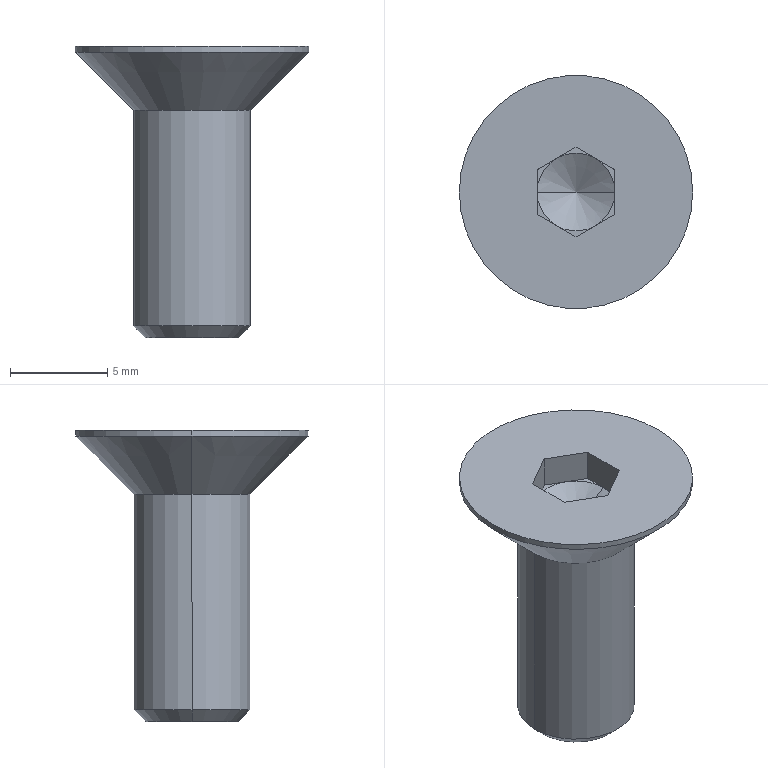Part | SolidWorks | features BaseBody 1 | 1 solid | 24 faces | box 12 x 12 x 15 mm | volume 531.654 mm3 | plane 14 | cone 6 | cylinder 4 | commonest cylinder face diameters 6 x2 12 x2
STEP:
#1=CARTESIAN_POINT('',(3.,0.,-11.086));
#2=VERTEX_POINT('',#1);
#3=CARTESIAN_POINT('',(-3.,0.,-11.086));
#4=VERTEX_POINT('',#3);
#5=CARTESIAN_POINT('',(0.,0.,-11.086));
#6=DIRECTION('',(0.,0.,1.));
#7=DIRECTION('',(1.,0.,0.));
#8=AXIS2_PLACEMENT_3D('',#5,#6,#7);
#9=CIRCLE('',#8,3.);
#10=EDGE_CURVE('',#2,#4,#9,.T.);
#11=ORIENTED_EDGE('',*,*,#10,.T.);
#12=CARTESIAN_POINT('',(-3.,0.,0.));
#13=VERTEX_POINT('',#12);
#14=CARTESIAN_POINT('',(-3.,0.,-11.7));
#15=DIRECTION('',(0.,0.,1.));
#16=VECTOR('',#15,1000.);
#17=LINE('',#14,#16);
#18=EDGE_CURVE('',#4,#13,#17,.T.);
#19=ORIENTED_EDGE('',*,*,#18,.T.);
#20=CARTESIAN_POINT('',(3.,0.,0.));
#21=VERTEX_POINT('',#20);
#22=CARTESIAN_POINT('',(0.,0.,0.));
#23=DIRECTION('',(0.,0.,-1.));
#24=DIRECTION('',(1.,0.,0.));
#25=AXIS2_PLACEMENT_3D('',#22,#23,#24);
#26=CIRCLE('',#25,3.);
#27=EDGE_CURVE('',#13,#21,#26,.T.);
#28=ORIENTED_EDGE('',*,*,#27,.T.);
#29=CARTESIAN_POINT('',(3.,0.,-11.7));
#30=DIRECTION('',(0.,0.,1.));
#31=VECTOR('',#30,1000.);
#32=LINE('',#29,#31);
#33=EDGE_CURVE('',#2,#21,#32,.T.);
#34=ORIENTED_EDGE('',*,*,#33,.F.);
#35=EDGE_LOOP('',(#11,#19,#28,#34));
#36=FACE_OUTER_BOUND('',#35,.T.);
#37=CARTESIAN_POINT('',(0.,0.,-11.7));
#38=DIRECTION('',(0.,0.,1.));
#39=DIRECTION('',(1.,0.,0.));
#40=AXIS2_PLACEMENT_3D('',#37,#38,#39);
#41=CYLINDRICAL_SURFACE('',#40,3.);
#42=ADVANCED_FACE('',(#36),#41,.T.);
#43=ORIENTED_EDGE('',*,*,#27,.F.);
#44=CARTESIAN_POINT('',(-6.,0.,3.));
#45=VERTEX_POINT('',#44);
#46=CARTESIAN_POINT('',(-6.,0.,3.));
#47=DIRECTION('',(-0.7071,0.,0.7071));
#48=VECTOR('',#47,1000.);
#49=LINE('',#46,#48);
#50=EDGE_CURVE('',#13,#45,#49,.T.);
#51=ORIENTED_EDGE('',*,*,#50,.T.);
#52=CARTESIAN_POINT('',(6.,0.,3.));
#53=VERTEX_POINT('',#52);
#54=CARTESIAN_POINT('',(0.,0.,3.));
#55=DIRECTION('',(0.,0.,-1.));
#56=DIRECTION('',(1.,0.,0.));
#57=AXIS2_PLACEMENT_3D('',#54,#55,#56);
#58=CIRCLE('',#57,6.);
#59=EDGE_CURVE('',#45,#53,#58,.T.);
#60=ORIENTED_EDGE('',*,*,#59,.T.);
#61=CARTESIAN_POINT('',(6.,0.,3.));
#62=DIRECTION('',(0.7071,0.,0.7071));
#63=VECTOR('',#62,1000.);
#64=LINE('',#61,#63);
#65=EDGE_CURVE('',#21,#53,#64,.T.);
#66=ORIENTED_EDGE('',*,*,#65,.F.);
#67=EDGE_LOOP('',(#43,#51,#60,#66));
#68=FACE_OUTER_BOUND('',#67,.T.);
#69=CARTESIAN_POINT('',(0.,0.,3.));
#70=DIRECTION('',(0.,0.,1.));
#71=DIRECTION('',(1.,0.,0.));
#72=AXIS2_PLACEMENT_3D('',#69,#70,#71);
#73=CONICAL_SURFACE('',#72,6.,0.7854);
#74=ADVANCED_FACE('',(#68),#73,.T.);
#75=CARTESIAN_POINT('',(2.387,0.,-11.7));
#76=VERTEX_POINT('',#75);
#77=CARTESIAN_POINT('',(-2.387,0.,-11.7));
#78=VERTEX_POINT('',#77);
#79=CARTESIAN_POINT('',(0.,0.,-11.7));
#80=DIRECTION('',(0.,0.,1.));
#81=DIRECTION('',(1.,0.,0.));
#82=AXIS2_PLACEMENT_3D('',#79,#80,#81);
#83=CIRCLE('',#82,2.387);
#84=EDGE_CURVE('',#76,#78,#83,.T.);
#85=ORIENTED_EDGE('',*,*,#84,.T.);
#86=CARTESIAN_POINT('',(-3.,0.,-11.087));
#87=DIRECTION('',(-0.7071,0.,0.7071));
#88=VECTOR('',#87,1000.);
#89=LINE('',#86,#88);
#90=EDGE_CURVE('',#78,#4,#89,.T.);
#91=ORIENTED_EDGE('',*,*,#90,.T.);
#92=ORIENTED_EDGE('',*,*,#10,.F.);
#93=CARTESIAN_POINT('',(3.,0.,-11.087));
#94=DIRECTION('',(0.7071,0.,0.7071));
#95=VECTOR('',#94,1000.);
#96=LINE('',#93,#95);
#97=EDGE_CURVE('',#76,#2,#96,.T.);
#98=ORIENTED_EDGE('',*,*,#97,.F.);
#99=EDGE_LOOP('',(#85,#91,#92,#98));
#100=FACE_OUTER_BOUND('',#99,.T.);
#101=CARTESIAN_POINT('',(0.,0.,-11.087));
#102=DIRECTION('',(0.,0.,1.));
#103=DIRECTION('',(1.,0.,0.));
#104=AXIS2_PLACEMENT_3D('',#101,#102,#103);
#105=CONICAL_SURFACE('',#104,3.,0.7854);
#106=ADVANCED_FACE('',(#100),#105,.T.);
#107=ORIENTED_EDGE('',*,*,#59,.F.);
#108=CARTESIAN_POINT('',(-6.,0.,3.3));
#109=VERTEX_POINT('',#108);
#110=CARTESIAN_POINT('',(-6.,0.,0.));
#111=DIRECTION('',(0.,0.,1.));
#112=VECTOR('',#111,1000.);
#113=LINE('',#110,#112);
#114=EDGE_CURVE('',#45,#109,#113,.T.);
#115=ORIENTED_EDGE('',*,*,#114,.T.);
#116=CARTESIAN_POINT('',(6.,0.,3.3));
#117=VERTEX_POINT('',#116);
#118=CARTESIAN_POINT('',(0.,0.,3.3));
#119=DIRECTION('',(0.,0.,-1.));
#120=DIRECTION('',(1.,0.,0.));
#121=AXIS2_PLACEMENT_3D('',#118,#119,#120);
#122=CIRCLE('',#121,6.);
#123=EDGE_CURVE('',#109,#117,#122,.T.);
#124=ORIENTED_EDGE('',*,*,#123,.T.);
#125=CARTESIAN_POINT('',(6.,0.,0.));
#126=DIRECTION('',(0.,0.,1.));
#127=VECTOR('',#126,1000.);
#128=LINE('',#125,#127);
#129=EDGE_CURVE('',#53,#117,#128,.T.);
#130=ORIENTED_EDGE('',*,*,#129,.F.);
#131=EDGE_LOOP('',(#107,#115,#124,#130));
#132=FACE_OUTER_BOUND('',#131,.T.);
#133=CARTESIAN_POINT('',(0.,0.,0.));
#134=DIRECTION('',(0.,0.,1.));
#135=DIRECTION('',(1.,0.,0.));
#136=AXIS2_PLACEMENT_3D('',#133,#134,#135);
#137=CYLINDRICAL_SURFACE('',#136,6.);
#138=ADVANCED_FACE('',(#132),#137,.T.);
#139=CARTESIAN_POINT('',(0.,0.,0.4953));
#140=VERTEX_POINT('',#139);
#141=CARTESIAN_POINT('',(2.,0.,1.65));
#142=VERTEX_POINT('',#141);
#143=CARTESIAN_POINT('',(2.,0.,1.65));
#144=DIRECTION('',(0.866,0.,0.5));
#145=VECTOR('',#144,1000.);
#146=LINE('',#143,#145);
#147=EDGE_CURVE('',#140,#142,#146,.T.);
#148=ORIENTED_EDGE('',*,*,#147,.F.);
#149=CARTESIAN_POINT('',(-2.,0.,1.65));
#150=VERTEX_POINT('',#149);
#151=CARTESIAN_POINT('',(-2.,0.,1.65));
#152=DIRECTION('',(-0.866,0.,0.5));
#153=VECTOR('',#152,1000.);
#154=LINE('',#151,#153);
#155=EDGE_CURVE('',#140,#150,#154,.T.);
#156=ORIENTED_EDGE('',*,*,#155,.T.);
#157=CARTESIAN_POINT('',(-1.,-1.732,1.65));
#158=VERTEX_POINT('',#157);
#159=CARTESIAN_POINT('',(0.,0.,1.65));
#160=DIRECTION('',(0.,0.,-1.));
#161=DIRECTION('',(1.,0.,0.));
#162=AXIS2_PLACEMENT_3D('',#159,#160,#161);
#163=CIRCLE('',#162,2.);
#164=EDGE_CURVE('',#158,#150,#163,.T.);
#165=ORIENTED_EDGE('',*,*,#164,.F.);
#166=CARTESIAN_POINT('',(1.,-1.732,1.65));
#167=VERTEX_POINT('',#166);
#168=CARTESIAN_POINT('',(0.,0.,1.65));
#169=DIRECTION('',(0.,0.,-1.));
#170=DIRECTION('',(1.,0.,0.));
#171=AXIS2_PLACEMENT_3D('',#168,#169,#170);
#172=CIRCLE('',#171,2.);
#173=EDGE_CURVE('',#167,#158,#172,.T.);
#174=ORIENTED_EDGE('',*,*,#173,.F.);
#175=CARTESIAN_POINT('',(0.,0.,1.65));
#176=DIRECTION('',(0.,0.,-1.));
#177=DIRECTION('',(1.,0.,0.));
#178=AXIS2_PLACEMENT_3D('',#175,#176,#177);
#179=CIRCLE('',#178,2.);
#180=EDGE_CURVE('',#142,#167,#179,.T.);
#181=ORIENTED_EDGE('',*,*,#180,.F.);
#182=EDGE_LOOP('',(#148,#156,#165,#174,#181));
#183=FACE_OUTER_BOUND('',#182,.T.);
#184=CARTESIAN_POINT('',(0.,0.,1.65));
#185=DIRECTION('',(0.,0.,1.));
#186=DIRECTION('',(1.,0.,0.));
#187=AXIS2_PLACEMENT_3D('',#184,#185,#186);
#188=CONICAL_SURFACE('',#187,2.,1.047);
#189=ADVANCED_FACE('',(#183),#188,.F.);
#190=ORIENTED_EDGE('',*,*,#18,.F.);
#191=CARTESIAN_POINT('',(0.,0.,-11.086));
#192=DIRECTION('',(0.,0.,1.));
#193=DIRECTION('',(1.,0.,0.));
#194=AXIS2_PLACEMENT_3D('',#191,#192,#193);
#195=CIRCLE('',#194,3.);
#196=EDGE_CURVE('',#4,#2,#195,.T.);
#197=ORIENTED_EDGE('',*,*,#196,.T.);
#198=ORIENTED_EDGE('',*,*,#33,.T.);
#199=CARTESIAN_POINT('',(0.,0.,0.));
#200=DIRECTION('',(0.,0.,-1.));
#201=DIRECTION('',(1.,0.,0.));
#202=AXIS2_PLACEMENT_3D('',#199,#200,#201);
#203=CIRCLE('',#202,3.);
#204=EDGE_CURVE('',#21,#13,#203,.T.);
#205=ORIENTED_EDGE('',*,*,#204,.T.);
#206=EDGE_LOOP('',(#190,#197,#198,#205));
#207=FACE_OUTER_BOUND('',#206,.T.);
#208=CARTESIAN_POINT('',(0.,0.,-11.7));
#209=DIRECTION('',(0.,0.,1.));
#210=DIRECTION('',(1.,0.,0.));
#211=AXIS2_PLACEMENT_3D('',#208,#209,#210);
#212=CYLINDRICAL_SURFACE('',#211,3.);
#213=ADVANCED_FACE('',(#207),#212,.T.);
#214=ORIENTED_EDGE('',*,*,#50,.F.);
#215=ORIENTED_EDGE('',*,*,#204,.F.);
#216=ORIENTED_EDGE('',*,*,#65,.T.);
#217=CARTESIAN_POINT('',(0.,0.,3.));
#218=DIRECTION('',(0.,0.,-1.));
#219=DIRECTION('',(1.,0.,0.));
#220=AXIS2_PLACEMENT_3D('',#217,#218,#219);
#221=CIRCLE('',#220,6.);
#222=EDGE_CURVE('',#53,#45,#221,.T.);
#223=ORIENTED_EDGE('',*,*,#222,.T.);
#224=EDGE_LOOP('',(#214,#215,#216,#223));
#225=FACE_OUTER_BOUND('',#224,.T.);
#226=CARTESIAN_POINT('',(0.,0.,3.));
#227=DIRECTION('',(0.,0.,1.));
#228=DIRECTION('',(1.,0.,0.));
#229=AXIS2_PLACEMENT_3D('',#226,#227,#228);
#230=CONICAL_SURFACE('',#229,6.,0.7854);
#231=ADVANCED_FACE('',(#225),#230,.T.);
#232=ORIENTED_EDGE('',*,*,#90,.F.);
#233=CARTESIAN_POINT('',(0.,0.,-11.7));
#234=DIRECTION('',(0.,0.,1.));
#235=DIRECTION('',(1.,0.,0.));
#236=AXIS2_PLACEMENT_3D('',#233,#234,#235);
#237=CIRCLE('',#236,2.387);
#238=EDGE_CURVE('',#78,#76,#237,.T.);
#239=ORIENTED_EDGE('',*,*,#238,.T.);
#240=ORIENTED_EDGE('',*,*,#97,.T.);
#241=ORIENTED_EDGE('',*,*,#196,.F.);
#242=EDGE_LOOP('',(#232,#239,#240,#241));
#243=FACE_OUTER_BOUND('',#242,.T.);
#244=CARTESIAN_POINT('',(0.,0.,-11.087));
#245=DIRECTION('',(0.,0.,1.));
#246=DIRECTION('',(1.,0.,0.));
#247=AXIS2_PLACEMENT_3D('',#244,#245,#246);
#248=CONICAL_SURFACE('',#247,3.,0.7854);
#249=ADVANCED_FACE('',(#243),#248,.T.);
#250=ORIENTED_EDGE('',*,*,#114,.F.);
#251=ORIENTED_EDGE('',*,*,#222,.F.);
#252=ORIENTED_EDGE('',*,*,#129,.T.);
#253=CARTESIAN_POINT('',(0.,0.,3.3));
#254=DIRECTION('',(0.,0.,-1.));
#255=DIRECTION('',(1.,0.,0.));
#256=AXIS2_PLACEMENT_3D('',#253,#254,#255);
#257=CIRCLE('',#256,6.);
#258=EDGE_CURVE('',#117,#109,#257,.T.);
#259=ORIENTED_EDGE('',*,*,#258,.T.);
#260=EDGE_LOOP('',(#250,#251,#252,#259));
#261=FACE_OUTER_BOUND('',#260,.T.);
#262=CARTESIAN_POINT('',(0.,0.,0.));
#263=DIRECTION('',(0.,0.,1.));
#264=DIRECTION('',(1.,0.,0.));
#265=AXIS2_PLACEMENT_3D('',#262,#263,#264);
#266=CYLINDRICAL_SURFACE('',#265,6.);
#267=ADVANCED_FACE('',(#261),#266,.T.);
#268=ORIENTED_EDGE('',*,*,#84,.F.);
#269=ORIENTED_EDGE('',*,*,#238,.F.);
#270=EDGE_LOOP('',(#268,#269));
#271=FACE_OUTER_BOUND('',#270,.T.);
#272=CARTESIAN_POINT('',(0.,2.386,-11.7));
#273=DIRECTION('',(0.,0.,1.));
#274=DIRECTION('',(1.,0.,0.));
#275=AXIS2_PLACEMENT_3D('',#272,#273,#274);
#276=PLANE('',#275);
#277=ADVANCED_FACE('',(#271),#276,.F.);
#278=CARTESIAN_POINT('',(-2.,-1.155,3.3));
#279=VERTEX_POINT('',#278);
#280=CARTESIAN_POINT('',(0.,-2.309,3.3));
#281=VERTEX_POINT('',#280);
#282=CARTESIAN_POINT('',(-2.,-1.155,3.3));
#283=DIRECTION('',(0.866,-0.5,0.));
#284=VECTOR('',#283,1000.);
#285=LINE('',#282,#284);
#286=EDGE_CURVE('',#279,#281,#285,.T.);
#287=ORIENTED_EDGE('',*,*,#286,.F.);
#288=CARTESIAN_POINT('',(-2.,1.155,3.3));
#289=VERTEX_POINT('',#288);
#290=CARTESIAN_POINT('',(-2.,0.,3.3));
#291=DIRECTION('',(0.,-1.,0.));
#292=VECTOR('',#291,1000.);
#293=LINE('',#290,#292);
#294=EDGE_CURVE('',#289,#279,#293,.T.);
#295=ORIENTED_EDGE('',*,*,#294,.F.);
#296=CARTESIAN_POINT('',(0.,2.309,3.3));
#297=VERTEX_POINT('',#296);
#298=CARTESIAN_POINT('',(0.,2.309,3.3));
#299=DIRECTION('',(-0.866,-0.5,0.));
#300=VECTOR('',#299,1000.);
#301=LINE('',#298,#300);
#302=EDGE_CURVE('',#297,#289,#301,.T.);
#303=ORIENTED_EDGE('',*,*,#302,.F.);
#304=CARTESIAN_POINT('',(2.,1.155,3.3));
#305=VERTEX_POINT('',#304);
#306=CARTESIAN_POINT('',(2.,1.155,3.3));
#307=DIRECTION('',(-0.866,0.5,0.));
#308=VECTOR('',#307,1000.);
#309=LINE('',#306,#308);
#310=EDGE_CURVE('',#305,#297,#309,.T.);
#311=ORIENTED_EDGE('',*,*,#310,.F.);
#312=CARTESIAN_POINT('',(2.,-1.155,3.3));
#313=VERTEX_POINT('',#312);
#314=CARTESIAN_POINT('',(2.,0.,3.3));
#315=DIRECTION('',(0.,1.,0.));
#316=VECTOR('',#315,1000.);
#317=LINE('',#314,#316);
#318=EDGE_CURVE('',#313,#305,#317,.T.);
#319=ORIENTED_EDGE('',*,*,#318,.F.);
#320=CARTESIAN_POINT('',(0.,-2.309,3.3));
#321=DIRECTION('',(0.866,0.5,0.));
#322=VECTOR('',#321,1000.);
#323=LINE('',#320,#322);
#324=EDGE_CURVE('',#281,#313,#323,.T.);
#325=ORIENTED_EDGE('',*,*,#324,.F.);
#326=EDGE_LOOP('',(#287,#295,#303,#311,#319,#325));
#327=FACE_BOUND('',#326,.T.);
#328=ORIENTED_EDGE('',*,*,#258,.F.);
#329=ORIENTED_EDGE('',*,*,#123,.F.);
#330=EDGE_LOOP('',(#328,#329));
#331=FACE_OUTER_BOUND('',#330,.T.);
#332=CARTESIAN_POINT('',(0.,0.,3.3));
#333=DIRECTION('',(0.,0.,-1.));
#334=DIRECTION('',(-1.,0.,0.));
#335=AXIS2_PLACEMENT_3D('',#332,#333,#334);
#336=PLANE('',#335);
#337=ADVANCED_FACE('',(#327,#331),#336,.F.);
#338=CARTESIAN_POINT('',(2.,-1.155,1.65));
#339=VERTEX_POINT('',#338);
#340=CARTESIAN_POINT('',(2.,-1.155,1.65));
#341=DIRECTION('',(0.,0.,1.));
#342=VECTOR('',#341,1000.);
#343=LINE('',#340,#342);
#344=EDGE_CURVE('',#339,#313,#343,.T.);
#345=ORIENTED_EDGE('',*,*,#344,.F.);
#346=CARTESIAN_POINT('',(0.,-2.309,1.65));
#347=DIRECTION('',(0.866,0.5,0.));
#348=VECTOR('',#347,1000.);
#349=LINE('',#346,#348);
#350=EDGE_CURVE('',#167,#339,#349,.T.);
#351=ORIENTED_EDGE('',*,*,#350,.F.);
#352=CARTESIAN_POINT('',(0.,-2.309,1.65));
#353=VERTEX_POINT('',#352);
#354=CARTESIAN_POINT('',(0.,-2.309,1.65));
#355=DIRECTION('',(0.866,0.5,0.));
#356=VECTOR('',#355,1000.);
#357=LINE('',#354,#356);
#358=EDGE_CURVE('',#353,#167,#357,.T.);
#359=ORIENTED_EDGE('',*,*,#358,.F.);
#360=CARTESIAN_POINT('',(0.,-2.309,1.65));
#361=DIRECTION('',(0.,0.,-1.));
#362=VECTOR('',#361,1000.);
#363=LINE('',#360,#362);
#364=EDGE_CURVE('',#281,#353,#363,.T.);
#365=ORIENTED_EDGE('',*,*,#364,.F.);
#366=ORIENTED_EDGE('',*,*,#324,.T.);
#367=EDGE_LOOP('',(#345,#351,#359,#365,#366));
#368=FACE_OUTER_BOUND('',#367,.T.);
#369=CARTESIAN_POINT('',(0.,-2.309,1.65));
#370=DIRECTION('',(0.5,-0.866,0.));
#371=DIRECTION('',(0.866,0.5,0.));
#372=AXIS2_PLACEMENT_3D('',#369,#370,#371);
#373=PLANE('',#372);
#374=ADVANCED_FACE('',(#368),#373,.F.);
#375=ORIENTED_EDGE('',*,*,#364,.T.);
#376=CARTESIAN_POINT('',(-1.,-1.732,1.65));
#377=DIRECTION('',(0.866,-0.5,0.));
#378=VECTOR('',#377,1000.);
#379=LINE('',#376,#378);
#380=EDGE_CURVE('',#158,#353,#379,.T.);
#381=ORIENTED_EDGE('',*,*,#380,.F.);
#382=CARTESIAN_POINT('',(-2.,-1.155,1.65));
#383=VERTEX_POINT('',#382);
#384=CARTESIAN_POINT('',(-2.,-1.155,1.65));
#385=DIRECTION('',(0.866,-0.5,0.));
#386=VECTOR('',#385,1000.);
#387=LINE('',#384,#386);
#388=EDGE_CURVE('',#383,#158,#387,.T.);
#389=ORIENTED_EDGE('',*,*,#388,.F.);
#390=CARTESIAN_POINT('',(-2.,-1.155,1.65));
#391=DIRECTION('',(0.,0.,-1.));
#392=VECTOR('',#391,1000.);
#393=LINE('',#390,#392);
#394=EDGE_CURVE('',#279,#383,#393,.T.);
#395=ORIENTED_EDGE('',*,*,#394,.F.);
#396=ORIENTED_EDGE('',*,*,#286,.T.);
#397=EDGE_LOOP('',(#375,#381,#389,#395,#396));
#398=FACE_OUTER_BOUND('',#397,.T.);
#399=CARTESIAN_POINT('',(-2.,-1.155,1.65));
#400=DIRECTION('',(-0.5,-0.866,0.));
#401=DIRECTION('',(0.866,-0.5,0.));
#402=AXIS2_PLACEMENT_3D('',#399,#400,#401);
#403=PLANE('',#402);
#404=ADVANCED_FACE('',(#398),#403,.F.);
#405=ORIENTED_EDGE('',*,*,#394,.T.);
#406=CARTESIAN_POINT('',(-2.,0.,1.65));
#407=DIRECTION('',(0.,-1.,0.));
#408=VECTOR('',#407,1000.);
#409=LINE('',#406,#408);
#410=EDGE_CURVE('',#150,#383,#409,.T.);
#411=ORIENTED_EDGE('',*,*,#410,.F.);
#412=CARTESIAN_POINT('',(-2.,1.155,1.65));
#413=VERTEX_POINT('',#412);
#414=CARTESIAN_POINT('',(-2.,0.,1.65));
#415=DIRECTION('',(0.,-1.,0.));
#416=VECTOR('',#415,1000.);
#417=LINE('',#414,#416);
#418=EDGE_CURVE('',#413,#150,#417,.T.);
#419=ORIENTED_EDGE('',*,*,#418,.F.);
#420=CARTESIAN_POINT('',(-2.,1.155,1.65));
#421=DIRECTION('',(0.,0.,-1.));
#422=VECTOR('',#421,1000.);
#423=LINE('',#420,#422);
#424=EDGE_CURVE('',#289,#413,#423,.T.);
#425=ORIENTED_EDGE('',*,*,#424,.F.);
#426=ORIENTED_EDGE('',*,*,#294,.T.);
#427=EDGE_LOOP('',(#405,#411,#419,#425,#426));
#428=FACE_OUTER_BOUND('',#427,.T.);
#429=CARTESIAN_POINT('',(-2.,1.155,1.65));
#430=DIRECTION('',(-1.,0.,0.));
#431=DIRECTION('',(0.,0.,1.));
#432=AXIS2_PLACEMENT_3D('',#429,#430,#431);
#433=PLANE('',#432);
#434=ADVANCED_FACE('',(#428),#433,.F.);
#435=ORIENTED_EDGE('',*,*,#424,.T.);
#436=CARTESIAN_POINT('',(-1.,1.732,1.65));
#437=VERTEX_POINT('',#436);
#438=CARTESIAN_POINT('',(-1.,1.732,1.65));
#439=DIRECTION('',(-0.866,-0.5,0.));
#440=VECTOR('',#439,1000.);
#441=LINE('',#438,#440);
#442=EDGE_CURVE('',#437,#413,#441,.T.);
#443=ORIENTED_EDGE('',*,*,#442,.F.);
#444=CARTESIAN_POINT('',(0.,2.309,1.65));
#445=VERTEX_POINT('',#444);
#446=CARTESIAN_POINT('',(0.,2.309,1.65));
#447=DIRECTION('',(-0.866,-0.5,0.));
#448=VECTOR('',#447,1000.);
#449=LINE('',#446,#448);
#450=EDGE_CURVE('',#445,#437,#449,.T.);
#451=ORIENTED_EDGE('',*,*,#450,.F.);
#452=CARTESIAN_POINT('',(0.,2.309,1.65));
#453=DIRECTION('',(0.,0.,-1.));
#454=VECTOR('',#453,1000.);
#455=LINE('',#452,#454);
#456=EDGE_CURVE('',#297,#445,#455,.T.);
#457=ORIENTED_EDGE('',*,*,#456,.F.);
#458=ORIENTED_EDGE('',*,*,#302,.T.);
#459=EDGE_LOOP('',(#435,#443,#451,#457,#458));
#460=FACE_OUTER_BOUND('',#459,.T.);
#461=CARTESIAN_POINT('',(0.,2.309,1.65));
#462=DIRECTION('',(-0.5,0.866,0.));
#463=DIRECTION('',(-0.866,-0.5,0.));
#464=AXIS2_PLACEMENT_3D('',#461,#462,#463);
#465=PLANE('',#464);
#466=ADVANCED_FACE('',(#460),#465,.F.);
#467=ORIENTED_EDGE('',*,*,#456,.T.);
#468=CARTESIAN_POINT('',(1.,1.732,1.65));
#469=VERTEX_POINT('',#468);
#470=CARTESIAN_POINT('',(1.,1.732,1.65));
#471=DIRECTION('',(-0.866,0.5,0.));
#472=VECTOR('',#471,1000.);
#473=LINE('',#470,#472);
#474=EDGE_CURVE('',#469,#445,#473,.T.);
#475=ORIENTED_EDGE('',*,*,#474,.F.);
#476=CARTESIAN_POINT('',(2.,1.155,1.65));
#477=VERTEX_POINT('',#476);
#478=CARTESIAN_POINT('',(2.,1.155,1.65));
#479=DIRECTION('',(-0.866,0.5,0.));
#480=VECTOR('',#479,1000.);
#481=LINE('',#478,#480);
#482=EDGE_CURVE('',#477,#469,#481,.T.);
#483=ORIENTED_EDGE('',*,*,#482,.F.);
#484=CARTESIAN_POINT('',(2.,1.155,1.65));
#485=DIRECTION('',(0.,0.,-1.));
#486=VECTOR('',#485,1000.);
#487=LINE('',#484,#486);
#488=EDGE_CURVE('',#305,#477,#487,.T.);
#489=ORIENTED_EDGE('',*,*,#488,.F.);
#490=ORIENTED_EDGE('',*,*,#310,.T.);
#491=EDGE_LOOP('',(#467,#475,#483,#489,#490));
#492=FACE_OUTER_BOUND('',#491,.T.);
#493=CARTESIAN_POINT('',(2.,1.155,1.65));
#494=DIRECTION('',(0.5,0.866,0.));
#495=DIRECTION('',(-0.866,0.5,0.));
#496=AXIS2_PLACEMENT_3D('',#493,#494,#495);
#497=PLANE('',#496);
#498=ADVANCED_FACE('',(#492),#497,.F.);
#499=ORIENTED_EDGE('',*,*,#488,.T.);
#500=CARTESIAN_POINT('',(2.,0.,1.65));
#501=DIRECTION('',(0.,1.,0.));
#502=VECTOR('',#501,1000.);
#503=LINE('',#500,#502);
#504=EDGE_CURVE('',#142,#477,#503,.T.);
#505=ORIENTED_EDGE('',*,*,#504,.F.);
#506=CARTESIAN_POINT('',(2.,-1.155,1.65));
#507=DIRECTION('',(0.,1.,0.));
#508=VECTOR('',#507,1000.);
#509=LINE('',#506,#508);
#510=EDGE_CURVE('',#339,#142,#509,.T.);
#511=ORIENTED_EDGE('',*,*,#510,.F.);
#512=ORIENTED_EDGE('',*,*,#344,.T.);
#513=ORIENTED_EDGE('',*,*,#318,.T.);
#514=EDGE_LOOP('',(#499,#505,#511,#512,#513));
#515=FACE_OUTER_BOUND('',#514,.T.);
#516=CARTESIAN_POINT('',(2.,-1.155,1.65));
#517=DIRECTION('',(1.,0.,0.));
#518=DIRECTION('',(0.,0.,-1.));
#519=AXIS2_PLACEMENT_3D('',#516,#517,#518);
#520=PLANE('',#519);
#521=ADVANCED_FACE('',(#515),#520,.F.);
#522=ORIENTED_EDGE('',*,*,#180,.T.);
#523=ORIENTED_EDGE('',*,*,#350,.T.);
#524=ORIENTED_EDGE('',*,*,#510,.T.);
#525=EDGE_LOOP('',(#522,#523,#524));
#526=FACE_OUTER_BOUND('',#525,.T.);
#527=CARTESIAN_POINT('',(0.,0.,1.65));
#528=DIRECTION('',(0.,0.,1.));
#529=DIRECTION('',(1.,0.,0.));
#530=AXIS2_PLACEMENT_3D('',#527,#528,#529);
#531=PLANE('',#530);
#532=ADVANCED_FACE('',(#526),#531,.T.);
#533=ORIENTED_EDGE('',*,*,#155,.F.);
#534=ORIENTED_EDGE('',*,*,#147,.T.);
#535=CARTESIAN_POINT('',(0.,0.,1.65));
#536=DIRECTION('',(0.,0.,-1.));
#537=DIRECTION('',(1.,0.,0.));
#538=AXIS2_PLACEMENT_3D('',#535,#536,#537);
#539=CIRCLE('',#538,2.);
#540=EDGE_CURVE('',#469,#142,#539,.T.);
#541=ORIENTED_EDGE('',*,*,#540,.F.);
#542=CARTESIAN_POINT('',(0.,0.,1.65));
#543=DIRECTION('',(0.,0.,-1.));
#544=DIRECTION('',(1.,0.,0.));
#545=AXIS2_PLACEMENT_3D('',#542,#543,#544);
#546=CIRCLE('',#545,2.);
#547=EDGE_CURVE('',#437,#469,#546,.T.);
#548=ORIENTED_EDGE('',*,*,#547,.F.);
#549=CARTESIAN_POINT('',(0.,0.,1.65));
#550=DIRECTION('',(0.,0.,-1.));
#551=DIRECTION('',(1.,0.,0.));
#552=AXIS2_PLACEMENT_3D('',#549,#550,#551);
#553=CIRCLE('',#552,2.);
#554=EDGE_CURVE('',#150,#437,#553,.T.);
#555=ORIENTED_EDGE('',*,*,#554,.F.);
#556=EDGE_LOOP('',(#533,#534,#541,#548,#555));
#557=FACE_OUTER_BOUND('',#556,.T.);
#558=CARTESIAN_POINT('',(0.,0.,1.65));
#559=DIRECTION('',(0.,0.,1.));
#560=DIRECTION('',(1.,0.,0.));
#561=AXIS2_PLACEMENT_3D('',#558,#559,#560);
#562=CONICAL_SURFACE('',#561,2.,1.047);
#563=ADVANCED_FACE('',(#557),#562,.F.);
#564=ORIENTED_EDGE('',*,*,#540,.T.);
#565=ORIENTED_EDGE('',*,*,#504,.T.);
#566=ORIENTED_EDGE('',*,*,#482,.T.);
#567=EDGE_LOOP('',(#564,#565,#566));
#568=FACE_OUTER_BOUND('',#567,.T.);
#569=CARTESIAN_POINT('',(0.,0.,1.65));
#570=DIRECTION('',(0.,0.,1.));
#571=DIRECTION('',(1.,0.,0.));
#572=AXIS2_PLACEMENT_3D('',#569,#570,#571);
#573=PLANE('',#572);
#574=ADVANCED_FACE('',(#568),#573,.T.);
#575=ORIENTED_EDGE('',*,*,#547,.T.);
#576=ORIENTED_EDGE('',*,*,#474,.T.);
#577=ORIENTED_EDGE('',*,*,#450,.T.);
#578=EDGE_LOOP('',(#575,#576,#577));
#579=FACE_OUTER_BOUND('',#578,.T.);
#580=CARTESIAN_POINT('',(0.,0.,1.65));
#581=DIRECTION('',(0.,0.,1.));
#582=DIRECTION('',(1.,0.,0.));
#583=AXIS2_PLACEMENT_3D('',#580,#581,#582);
#584=PLANE('',#583);
#585=ADVANCED_FACE('',(#579),#584,.T.);
#586=ORIENTED_EDGE('',*,*,#554,.T.);
#587=ORIENTED_EDGE('',*,*,#442,.T.);
#588=ORIENTED_EDGE('',*,*,#418,.T.);
#589=EDGE_LOOP('',(#586,#587,#588));
#590=FACE_OUTER_BOUND('',#589,.T.);
#591=CARTESIAN_POINT('',(0.,0.,1.65));
#592=DIRECTION('',(0.,0.,1.));
#593=DIRECTION('',(1.,0.,0.));
#594=AXIS2_PLACEMENT_3D('',#591,#592,#593);
#595=PLANE('',#594);
#596=ADVANCED_FACE('',(#590),#595,.T.);
#597=ORIENTED_EDGE('',*,*,#164,.T.);
#598=ORIENTED_EDGE('',*,*,#410,.T.);
#599=ORIENTED_EDGE('',*,*,#388,.T.);
#600=EDGE_LOOP('',(#597,#598,#599));
#601=FACE_OUTER_BOUND('',#600,.T.);
#602=CARTESIAN_POINT('',(0.,0.,1.65));
#603=DIRECTION('',(0.,0.,1.));
#604=DIRECTION('',(1.,0.,0.));
#605=AXIS2_PLACEMENT_3D('',#602,#603,#604);
#606=PLANE('',#605);
#607=ADVANCED_FACE('',(#601),#606,.T.);
#608=ORIENTED_EDGE('',*,*,#173,.T.);
#609=ORIENTED_EDGE('',*,*,#380,.T.);
#610=ORIENTED_EDGE('',*,*,#358,.T.);
#611=EDGE_LOOP('',(#608,#609,#610));
#612=FACE_OUTER_BOUND('',#611,.T.);
#613=CARTESIAN_POINT('',(0.,0.,1.65));
#614=DIRECTION('',(0.,0.,1.));
#615=DIRECTION('',(1.,0.,0.));
#616=AXIS2_PLACEMENT_3D('',#613,#614,#615);
#617=PLANE('',#616);
#618=ADVANCED_FACE('',(#612),#617,.T.);
#619=CLOSED_SHELL('',(#42,#74,#106,#138,#189,#213,#231,#249,#267,#277,#337,#374,#404,#434,#466,#498,#521,#532,#563,#574,#585,#596,#607,#618));
#620=MANIFOLD_SOLID_BREP('',#619);
#621=CARTESIAN_POINT('',(0.,0.,0.));
#622=DIRECTION('',(0.,0.,1.));
#623=DIRECTION('',(1.,0.,0.));
#624=AXIS2_PLACEMENT_3D('',#621,#622,#623);
#625=(LENGTH_UNIT()NAMED_UNIT(*)SI_UNIT(.MILLI.,.METRE.));
#626=UNCERTAINTY_MEASURE_WITH_UNIT(LENGTH_MEASURE(0.00001),#625,'','');
#627=(NAMED_UNIT(*)PLANE_ANGLE_UNIT()SI_UNIT($,.RADIAN.));
#628=(NAMED_UNIT(*)SI_UNIT($,.STERADIAN.)SOLID_ANGLE_UNIT());
#629=(GEOMETRIC_REPRESENTATION_CONTEXT(3)GLOBAL_UNCERTAINTY_ASSIGNED_CONTEXT((#626))GLOBAL_UNIT_ASSIGNED_CONTEXT((#625,#627,#628))REPRESENTATION_CONTEXT('',''));
#630=ADVANCED_BREP_SHAPE_REPRESENTATION('',(#620,#624),#629);